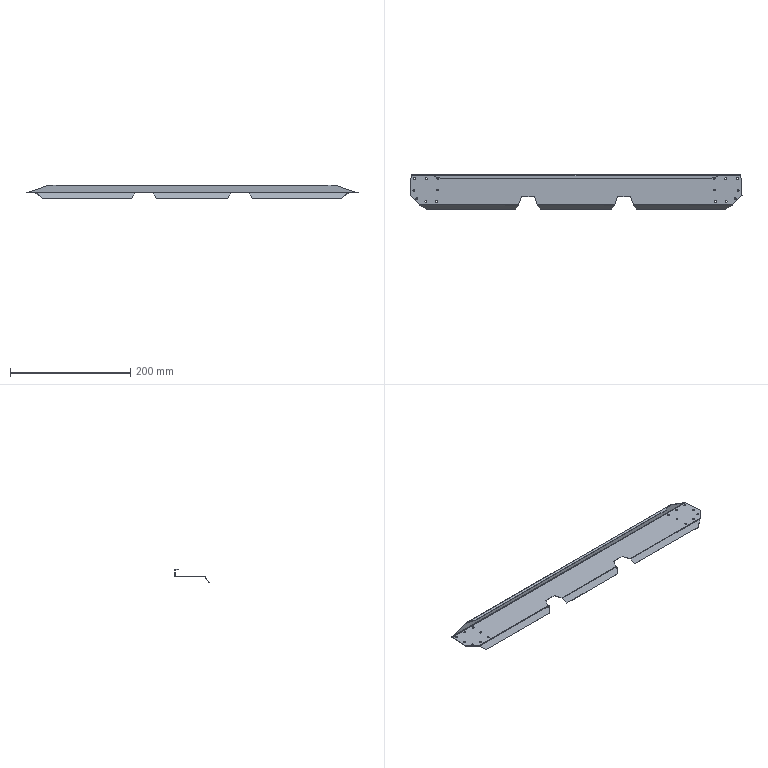Part | SolidWorks | features BaseBody 1 | 1 solid | 90 faces | box 552.944 x 56.791 x 22.498 mm | volume 20108 mm3 | cylinder 42 | plane 36 | spline 12 | commonest cylinder face diameters 3.2 x32 1.5 x3 2.5 x3 1 x2 2 x2